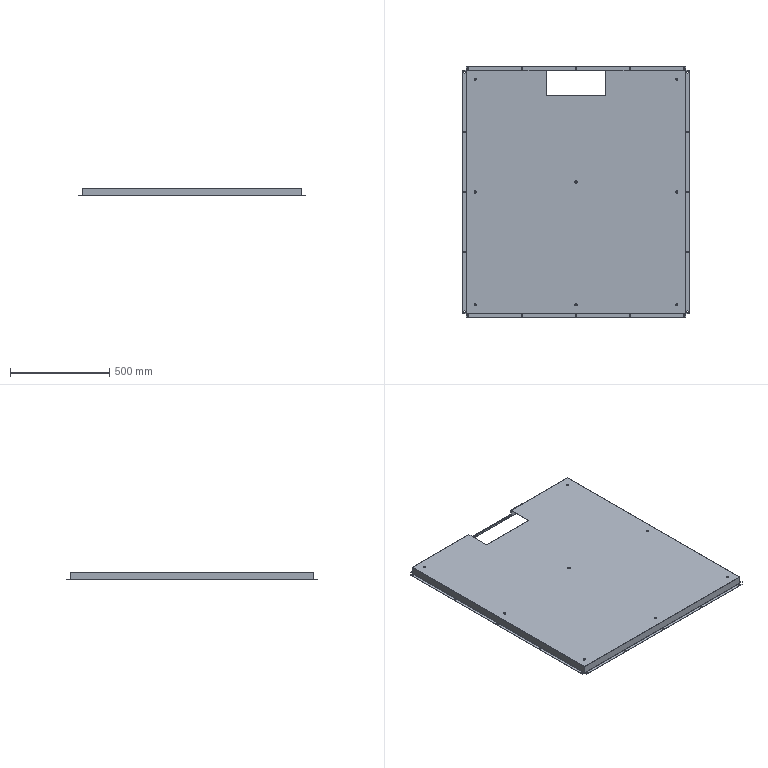Part | SolidWorks | features ICE 4, EdgeFlange 2, Cut 1, FlatPattern 1, SMBaseFlange 1, SheetMetal 1 | 1 solid | 186 faces | box 1139 x 1259 x 40 mm | volume 1562312 mm3 | plane 94 | cylinder 84 | spline 8 | commonest cylinder face diameters 7 x50 11 x16 0.4 x9 2.4 x9